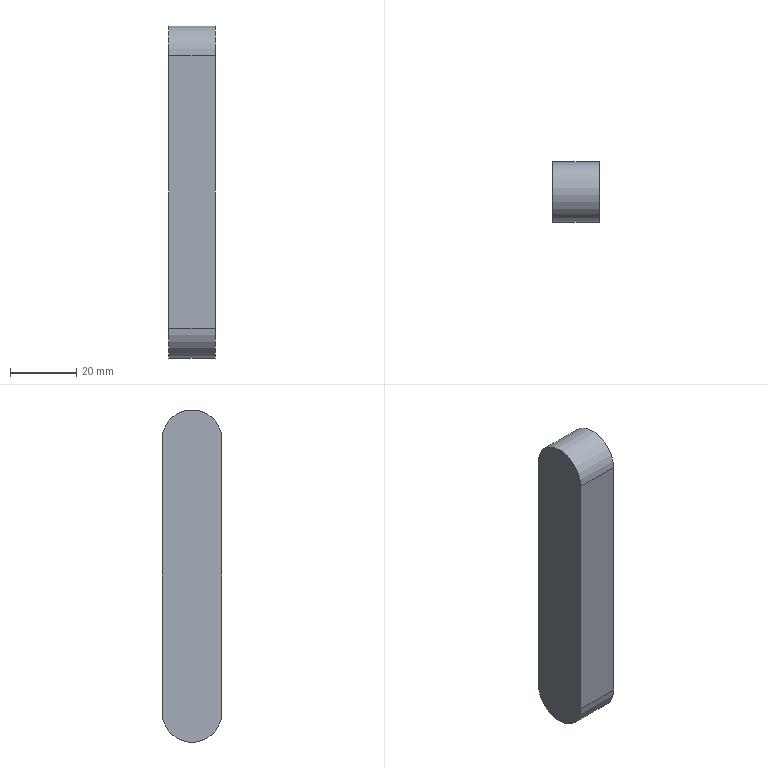Part | NX | 1 solid | 6 faces | box 14 x 18 x 100 mm | volume 24227 mm3 | plane 4 | cylinder 2 | commonest cylinder face diameters 18 x2
STEP:
#1=CARTESIAN_POINT('',(0.,-9.,41.));
#2=VERTEX_POINT('',#1);
#3=CARTESIAN_POINT('',(0.,-9.,-41.));
#4=VERTEX_POINT('',#3);
#5=CARTESIAN_POINT('',(0.,-9.,50.));
#6=DIRECTION('',(0.,0.,-1.));
#7=VECTOR('',#6,1.);
#8=LINE('',#5,#7);
#9=EDGE_CURVE('',#2,#4,#8,.T.);
#10=ORIENTED_EDGE('',*,*,#9,.T.);
#11=CARTESIAN_POINT('',(14.,-9.,-41.));
#12=VERTEX_POINT('',#11);
#13=CARTESIAN_POINT('',(14.,-9.,-41.));
#14=DIRECTION('',(1.,0.,0.));
#15=VECTOR('',#14,1.);
#16=LINE('',#13,#15);
#17=EDGE_CURVE('',#4,#12,#16,.T.);
#18=ORIENTED_EDGE('',*,*,#17,.T.);
#19=CARTESIAN_POINT('',(14.,-9.,41.));
#20=VERTEX_POINT('',#19);
#21=CARTESIAN_POINT('',(14.,-9.,50.));
#22=DIRECTION('',(0.,0.,-1.));
#23=VECTOR('',#22,1.);
#24=LINE('',#21,#23);
#25=EDGE_CURVE('',#20,#12,#24,.T.);
#26=ORIENTED_EDGE('',*,*,#25,.F.);
#27=CARTESIAN_POINT('',(14.,-9.,41.));
#28=DIRECTION('',(-1.,0.,0.));
#29=VECTOR('',#28,1.);
#30=LINE('',#27,#29);
#31=EDGE_CURVE('',#20,#2,#30,.T.);
#32=ORIENTED_EDGE('',*,*,#31,.T.);
#33=EDGE_LOOP('',(#10,#18,#26,#32));
#34=FACE_OUTER_BOUND('',#33,.T.);
#35=CARTESIAN_POINT('',(14.,-9.,50.));
#36=DIRECTION('',(0.,1.,0.));
#37=DIRECTION('',(0.,0.,-1.));
#38=AXIS2_PLACEMENT_3D('',#35,#36,#37);
#39=PLANE('',#38);
#40=ADVANCED_FACE('',(#34),#39,.F.);
#41=CARTESIAN_POINT('',(14.,9.,-41.));
#42=VERTEX_POINT('',#41);
#43=CARTESIAN_POINT('',(14.,9.,41.));
#44=VERTEX_POINT('',#43);
#45=CARTESIAN_POINT('',(14.,9.,-50.));
#46=DIRECTION('',(0.,0.,1.));
#47=VECTOR('',#46,1.);
#48=LINE('',#45,#47);
#49=EDGE_CURVE('',#42,#44,#48,.T.);
#50=ORIENTED_EDGE('',*,*,#49,.F.);
#51=CARTESIAN_POINT('',(0.,9.,-41.));
#52=VERTEX_POINT('',#51);
#53=CARTESIAN_POINT('',(14.,9.,-41.));
#54=DIRECTION('',(-1.,0.,0.));
#55=VECTOR('',#54,1.);
#56=LINE('',#53,#55);
#57=EDGE_CURVE('',#42,#52,#56,.T.);
#58=ORIENTED_EDGE('',*,*,#57,.T.);
#59=CARTESIAN_POINT('',(0.,9.,41.));
#60=VERTEX_POINT('',#59);
#61=CARTESIAN_POINT('',(0.,9.,-50.));
#62=DIRECTION('',(0.,0.,1.));
#63=VECTOR('',#62,1.);
#64=LINE('',#61,#63);
#65=EDGE_CURVE('',#52,#60,#64,.T.);
#66=ORIENTED_EDGE('',*,*,#65,.T.);
#67=CARTESIAN_POINT('',(14.,9.,41.));
#68=DIRECTION('',(1.,0.,0.));
#69=VECTOR('',#68,1.);
#70=LINE('',#67,#69);
#71=EDGE_CURVE('',#60,#44,#70,.T.);
#72=ORIENTED_EDGE('',*,*,#71,.T.);
#73=EDGE_LOOP('',(#50,#58,#66,#72));
#74=FACE_OUTER_BOUND('',#73,.T.);
#75=CARTESIAN_POINT('',(14.,9.,-50.));
#76=DIRECTION('',(0.,-1.,0.));
#77=DIRECTION('',(0.,0.,1.));
#78=AXIS2_PLACEMENT_3D('',#75,#76,#77);
#79=PLANE('',#78);
#80=ADVANCED_FACE('',(#74),#79,.F.);
#81=ORIENTED_EDGE('',*,*,#25,.T.);
#82=CARTESIAN_POINT('',(14.,0.,-41.));
#83=DIRECTION('',(1.,0.,0.));
#84=DIRECTION('',(0.,0.,-1.));
#85=AXIS2_PLACEMENT_3D('',#82,#83,#84);
#86=CIRCLE('',#85,9.);
#87=EDGE_CURVE('',#12,#42,#86,.T.);
#88=ORIENTED_EDGE('',*,*,#87,.T.);
#89=ORIENTED_EDGE('',*,*,#49,.T.);
#90=CARTESIAN_POINT('',(14.,0.,41.));
#91=DIRECTION('',(1.,0.,0.));
#92=DIRECTION('',(0.,0.,-1.));
#93=AXIS2_PLACEMENT_3D('',#90,#91,#92);
#94=CIRCLE('',#93,9.);
#95=EDGE_CURVE('',#44,#20,#94,.T.);
#96=ORIENTED_EDGE('',*,*,#95,.T.);
#97=EDGE_LOOP('',(#81,#88,#89,#96));
#98=FACE_OUTER_BOUND('',#97,.T.);
#99=CARTESIAN_POINT('',(14.,0.,0.));
#100=DIRECTION('',(1.,0.,0.));
#101=DIRECTION('',(0.,0.,1.));
#102=AXIS2_PLACEMENT_3D('',#99,#100,#101);
#103=PLANE('',#102);
#104=ADVANCED_FACE('',(#98),#103,.T.);
#105=CARTESIAN_POINT('',(0.,0.,-41.));
#106=DIRECTION('',(-1.,0.,0.));
#107=DIRECTION('',(0.,0.,-1.));
#108=AXIS2_PLACEMENT_3D('',#105,#106,#107);
#109=CIRCLE('',#108,9.);
#110=EDGE_CURVE('',#52,#4,#109,.T.);
#111=ORIENTED_EDGE('',*,*,#110,.T.);
#112=ORIENTED_EDGE('',*,*,#9,.F.);
#113=CARTESIAN_POINT('',(0.,0.,41.));
#114=DIRECTION('',(-1.,0.,0.));
#115=DIRECTION('',(0.,0.,-1.));
#116=AXIS2_PLACEMENT_3D('',#113,#114,#115);
#117=CIRCLE('',#116,9.);
#118=EDGE_CURVE('',#2,#60,#117,.T.);
#119=ORIENTED_EDGE('',*,*,#118,.T.);
#120=ORIENTED_EDGE('',*,*,#65,.F.);
#121=EDGE_LOOP('',(#111,#112,#119,#120));
#122=FACE_OUTER_BOUND('',#121,.T.);
#123=CARTESIAN_POINT('',(0.,0.,0.));
#124=DIRECTION('',(1.,0.,0.));
#125=DIRECTION('',(0.,0.,1.));
#126=AXIS2_PLACEMENT_3D('',#123,#124,#125);
#127=PLANE('',#126);
#128=ADVANCED_FACE('',(#122),#127,.F.);
#129=ORIENTED_EDGE('',*,*,#57,.F.);
#130=ORIENTED_EDGE('',*,*,#87,.F.);
#131=ORIENTED_EDGE('',*,*,#17,.F.);
#132=ORIENTED_EDGE('',*,*,#110,.F.);
#133=EDGE_LOOP('',(#129,#130,#131,#132));
#134=FACE_OUTER_BOUND('',#133,.T.);
#135=CARTESIAN_POINT('',(14.,0.,-41.));
#136=DIRECTION('',(-1.,0.,0.));
#137=DIRECTION('',(0.,0.,-1.));
#138=AXIS2_PLACEMENT_3D('',#135,#136,#137);
#139=CYLINDRICAL_SURFACE('',#138,9.);
#140=ADVANCED_FACE('',(#134),#139,.T.);
#141=ORIENTED_EDGE('',*,*,#31,.F.);
#142=ORIENTED_EDGE('',*,*,#95,.F.);
#143=ORIENTED_EDGE('',*,*,#71,.F.);
#144=ORIENTED_EDGE('',*,*,#118,.F.);
#145=EDGE_LOOP('',(#141,#142,#143,#144));
#146=FACE_OUTER_BOUND('',#145,.T.);
#147=CARTESIAN_POINT('',(14.,0.,41.));
#148=DIRECTION('',(-1.,0.,0.));
#149=DIRECTION('',(0.,0.,-1.));
#150=AXIS2_PLACEMENT_3D('',#147,#148,#149);
#151=CYLINDRICAL_SURFACE('',#150,9.);
#152=ADVANCED_FACE('',(#146),#151,.T.);
#153=CLOSED_SHELL('',(#40,#80,#104,#128,#140,#152));
#154=MANIFOLD_SOLID_BREP('',#153);
#155=(LENGTH_UNIT()NAMED_UNIT(*)SI_UNIT(.MILLI.,.METRE.));
#156=UNCERTAINTY_MEASURE_WITH_UNIT(LENGTH_MEASURE(0.00002),#155,'','');
#157=(NAMED_UNIT(*)PLANE_ANGLE_UNIT()SI_UNIT($,.RADIAN.));
#158=PLANE_ANGLE_MEASURE_WITH_UNIT(PLANE_ANGLE_MEASURE(0.01745),#157);
#159=DIMENSIONAL_EXPONENTS(0.,0.,0.,0.,0.,0.,0.);
#160=(CONVERSION_BASED_UNIT('DEGREE',#158)NAMED_UNIT(#159)PLANE_ANGLE_UNIT());
#161=(NAMED_UNIT(*)SI_UNIT($,.STERADIAN.)SOLID_ANGLE_UNIT());
#162=(GEOMETRIC_REPRESENTATION_CONTEXT(3)GLOBAL_UNCERTAINTY_ASSIGNED_CONTEXT((#156))GLOBAL_UNIT_ASSIGNED_CONTEXT((#155,#160,#161))REPRESENTATION_CONTEXT('',''));
#163=ADVANCED_BREP_SHAPE_REPRESENTATION('',(#154),#162);